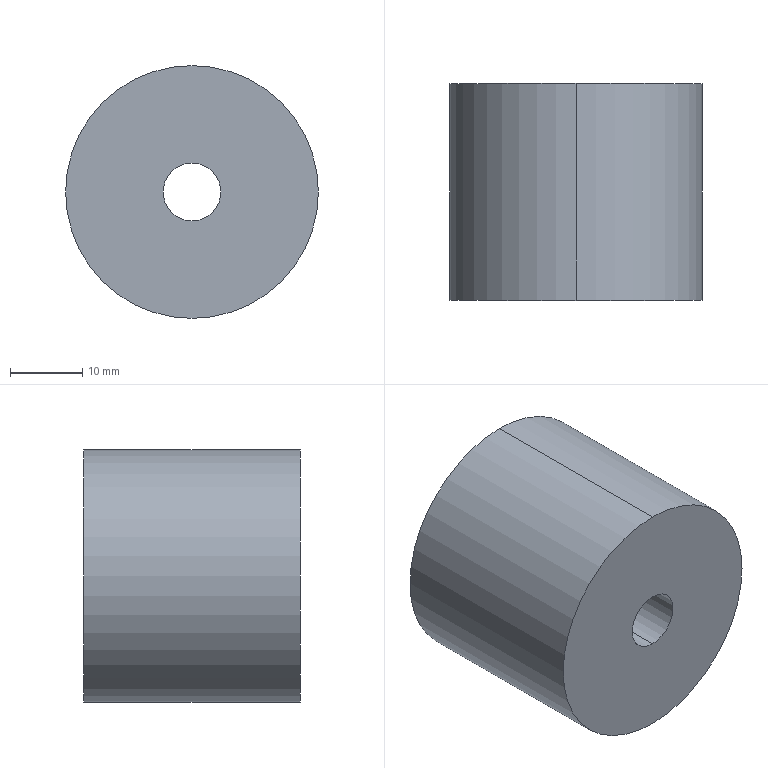Part | STEP file | Polyurethane anti-collision column 2 | 1 solid | 9 faces | box 35 x 30 x 35 mm | volume 26422 mm3 | cylinder 6 | plane 3 | commonest cylinder face diameters 8 x2 14 x2 35 x2
STEP:
#1=CARTESIAN_POINT('',(0.,0.,0.));
#2=DIRECTION('',(0.,0.,1.));
#3=DIRECTION('',(1.,0.,0.));
#4=AXIS2_PLACEMENT_3D('',#1,#2,#3);
#5=CARTESIAN_POINT('',(0.,21.,7.));
#6=VERTEX_POINT('',#5);
#7=CARTESIAN_POINT('',(0.,30.,7.));
#8=VERTEX_POINT('',#7);
#9=CARTESIAN_POINT('',(0.,30.,7.));
#10=DIRECTION('',(0.,1.,0.));
#11=VECTOR('',#10,1.);
#12=LINE('',#9,#11);
#13=CARTESIAN_POINT('',(0.,30.,0.));
#14=DIRECTION('',(0.,1.,0.));
#15=DIRECTION('',(0.,0.,1.));
#16=AXIS2_PLACEMENT_3D('',#13,#14,#15);
#17=CYLINDRICAL_SURFACE('',#16,7.);
#18=CARTESIAN_POINT('',(6.283,0.));
#19=DIRECTION('',(0.,1.));
#20=VECTOR('',#19,1.);
#21=LINE('',#18,#20);
#22=(GEOMETRIC_REPRESENTATION_CONTEXT(2)PARAMETRIC_REPRESENTATION_CONTEXT()REPRESENTATION_CONTEXT('',''));
#23=DEFINITIONAL_REPRESENTATION('',(#21),#22);
#24=PCURVE('',#17,#23);
#25=CARTESIAN_POINT('',(0.,30.,0.));
#26=DIRECTION('',(0.,1.,0.));
#27=DIRECTION('',(0.,0.,1.));
#28=AXIS2_PLACEMENT_3D('',#25,#26,#27);
#29=CYLINDRICAL_SURFACE('',#28,7.);
#30=CARTESIAN_POINT('',(0.,0.));
#31=DIRECTION('',(0.,1.));
#32=VECTOR('',#31,1.);
#33=LINE('',#30,#32);
#34=(GEOMETRIC_REPRESENTATION_CONTEXT(2)PARAMETRIC_REPRESENTATION_CONTEXT()REPRESENTATION_CONTEXT('',''));
#35=DEFINITIONAL_REPRESENTATION('',(#33),#34);
#36=PCURVE('',#29,#35);
#37=SURFACE_CURVE('',#12,(#24,#36),.PCURVE_S1.);
#38=EDGE_CURVE('',#6,#8,#37,.T.);
#39=ORIENTED_EDGE('',*,*,#38,.T.);
#40=CARTESIAN_POINT('',(0.,30.,-7.));
#41=VERTEX_POINT('',#40);
#42=CARTESIAN_POINT('',(0.,30.,0.));
#43=DIRECTION('',(0.,1.,0.));
#44=DIRECTION('',(0.,0.,1.));
#45=AXIS2_PLACEMENT_3D('',#42,#43,#44);
#46=CIRCLE('',#45,7.);
#47=CARTESIAN_POINT('',(0.,0.));
#48=DIRECTION('',(1.,0.));
#49=VECTOR('',#48,1.);
#50=LINE('',#47,#49);
#51=(GEOMETRIC_REPRESENTATION_CONTEXT(2)PARAMETRIC_REPRESENTATION_CONTEXT()REPRESENTATION_CONTEXT('',''));
#52=DEFINITIONAL_REPRESENTATION('',(#50),#51);
#53=PCURVE('',#17,#52);
#54=CARTESIAN_POINT('',(0.,30.,0.));
#55=DIRECTION('',(0.,1.,0.));
#56=DIRECTION('',(0.,0.,1.));
#57=AXIS2_PLACEMENT_3D('',#54,#55,#56);
#58=PLANE('',#57);
#59=CARTESIAN_POINT('',(0.,0.));
#60=DIRECTION('',(1.,0.));
#61=AXIS2_PLACEMENT_2D('',#59,#60);
#62=CIRCLE('',#61,7.);
#63=(GEOMETRIC_REPRESENTATION_CONTEXT(2)PARAMETRIC_REPRESENTATION_CONTEXT()REPRESENTATION_CONTEXT('',''));
#64=DEFINITIONAL_REPRESENTATION('',(#62),#63);
#65=PCURVE('',#58,#64);
#66=SURFACE_CURVE('',#46,(#53,#65),.PCURVE_S1.);
#67=EDGE_CURVE('',#41,#8,#66,.T.);
#68=ORIENTED_EDGE('',*,*,#67,.F.);
#69=CARTESIAN_POINT('',(0.,21.,-7.));
#70=VERTEX_POINT('',#69);
#71=CARTESIAN_POINT('',(0.,30.,-7.));
#72=DIRECTION('',(0.,1.,0.));
#73=VECTOR('',#72,1.);
#74=LINE('',#71,#73);
#75=CARTESIAN_POINT('',(3.142,0.));
#76=DIRECTION('',(0.,1.));
#77=VECTOR('',#76,1.);
#78=LINE('',#75,#77);
#79=(GEOMETRIC_REPRESENTATION_CONTEXT(2)PARAMETRIC_REPRESENTATION_CONTEXT()REPRESENTATION_CONTEXT('',''));
#80=DEFINITIONAL_REPRESENTATION('',(#78),#79);
#81=PCURVE('',#17,#80);
#82=CARTESIAN_POINT('',(3.142,0.));
#83=DIRECTION('',(0.,1.));
#84=VECTOR('',#83,1.);
#85=LINE('',#82,#84);
#86=(GEOMETRIC_REPRESENTATION_CONTEXT(2)PARAMETRIC_REPRESENTATION_CONTEXT()REPRESENTATION_CONTEXT('',''));
#87=DEFINITIONAL_REPRESENTATION('',(#85),#86);
#88=PCURVE('',#29,#87);
#89=SURFACE_CURVE('',#74,(#81,#88),.PCURVE_S1.);
#90=EDGE_CURVE('',#70,#41,#89,.T.);
#91=ORIENTED_EDGE('',*,*,#90,.F.);
#92=CARTESIAN_POINT('',(0.,21.,0.));
#93=DIRECTION('',(0.,1.,0.));
#94=DIRECTION('',(0.,0.,1.));
#95=AXIS2_PLACEMENT_3D('',#92,#93,#94);
#96=CIRCLE('',#95,7.);
#97=CARTESIAN_POINT('',(0.,-9.));
#98=DIRECTION('',(1.,0.));
#99=VECTOR('',#98,1.);
#100=LINE('',#97,#99);
#101=(GEOMETRIC_REPRESENTATION_CONTEXT(2)PARAMETRIC_REPRESENTATION_CONTEXT()REPRESENTATION_CONTEXT('',''));
#102=DEFINITIONAL_REPRESENTATION('',(#100),#101);
#103=PCURVE('',#17,#102);
#104=CARTESIAN_POINT('',(4.,21.,0.));
#105=DIRECTION('',(0.,-1.,0.));
#106=DIRECTION('',(0.,0.,-1.));
#107=AXIS2_PLACEMENT_3D('',#104,#105,#106);
#108=PLANE('',#107);
#109=CARTESIAN_POINT('',(-7.,-4.));
#110=CARTESIAN_POINT('',(-7.,8.124));
#111=CARTESIAN_POINT('',(3.5,2.062));
#112=CARTESIAN_POINT('',(14.,-4.));
#113=CARTESIAN_POINT('',(3.5,-10.062));
#114=CARTESIAN_POINT('',(-7.,-16.124));
#115=CARTESIAN_POINT('',(-7.,-4.));
#116=(BOUNDED_CURVE()B_SPLINE_CURVE(2,(#109,#110,#111,#112,#113,#114,#115),.UNSPECIFIED.,.T.,.F.)B_SPLINE_CURVE_WITH_KNOTS((1,2,2,2,2,1),(-2.094,0.,2.094,4.189,6.283,8.378),.UNSPECIFIED.)CURVE()GEOMETRIC_REPRESENTATION_ITEM()RATIONAL_B_SPLINE_CURVE((1.,0.5,1.,0.5,1.,0.5,1.))REPRESENTATION_ITEM(''));
#117=(GEOMETRIC_REPRESENTATION_CONTEXT(2)PARAMETRIC_REPRESENTATION_CONTEXT()REPRESENTATION_CONTEXT('',''));
#118=DEFINITIONAL_REPRESENTATION('',(#116),#117);
#119=PCURVE('',#108,#118);
#120=SURFACE_CURVE('',#96,(#103,#119),.PCURVE_S1.);
#121=EDGE_CURVE('',#70,#6,#120,.T.);
#122=ORIENTED_EDGE('',*,*,#121,.T.);
#123=EDGE_LOOP('',(#39,#68,#91,#122));
#124=FACE_BOUND('',#123,.F.);
#125=ADVANCED_FACE('',(#124),#17,.F.);
#126=CARTESIAN_POINT('',(0.,0.,4.));
#127=VERTEX_POINT('',#126);
#128=CARTESIAN_POINT('',(0.,21.,4.));
#129=VERTEX_POINT('',#128);
#130=CARTESIAN_POINT('',(0.,30.,4.));
#131=DIRECTION('',(0.,1.,0.));
#132=VECTOR('',#131,1.);
#133=LINE('',#130,#132);
#134=CARTESIAN_POINT('',(0.,30.,0.));
#135=DIRECTION('',(0.,1.,0.));
#136=DIRECTION('',(0.,0.,1.));
#137=AXIS2_PLACEMENT_3D('',#134,#135,#136);
#138=CYLINDRICAL_SURFACE('',#137,4.);
#139=CARTESIAN_POINT('',(6.283,0.));
#140=DIRECTION('',(0.,1.));
#141=VECTOR('',#140,1.);
#142=LINE('',#139,#141);
#143=(GEOMETRIC_REPRESENTATION_CONTEXT(2)PARAMETRIC_REPRESENTATION_CONTEXT()REPRESENTATION_CONTEXT('',''));
#144=DEFINITIONAL_REPRESENTATION('',(#142),#143);
#145=PCURVE('',#138,#144);
#146=CARTESIAN_POINT('',(0.,30.,0.));
#147=DIRECTION('',(0.,1.,0.));
#148=DIRECTION('',(0.,0.,1.));
#149=AXIS2_PLACEMENT_3D('',#146,#147,#148);
#150=CYLINDRICAL_SURFACE('',#149,4.);
#151=CARTESIAN_POINT('',(0.,0.));
#152=DIRECTION('',(0.,1.));
#153=VECTOR('',#152,1.);
#154=LINE('',#151,#153);
#155=(GEOMETRIC_REPRESENTATION_CONTEXT(2)PARAMETRIC_REPRESENTATION_CONTEXT()REPRESENTATION_CONTEXT('',''));
#156=DEFINITIONAL_REPRESENTATION('',(#154),#155);
#157=PCURVE('',#150,#156);
#158=SURFACE_CURVE('',#133,(#145,#157),.PCURVE_S1.);
#159=EDGE_CURVE('',#127,#129,#158,.T.);
#160=ORIENTED_EDGE('',*,*,#159,.T.);
#161=CARTESIAN_POINT('',(0.,21.,-4.));
#162=VERTEX_POINT('',#161);
#163=CARTESIAN_POINT('',(0.,21.,0.));
#164=DIRECTION('',(0.,1.,0.));
#165=DIRECTION('',(0.,0.,1.));
#166=AXIS2_PLACEMENT_3D('',#163,#164,#165);
#167=CIRCLE('',#166,4.);
#168=CARTESIAN_POINT('',(0.,-9.));
#169=DIRECTION('',(1.,0.));
#170=VECTOR('',#169,1.);
#171=LINE('',#168,#170);
#172=(GEOMETRIC_REPRESENTATION_CONTEXT(2)PARAMETRIC_REPRESENTATION_CONTEXT()REPRESENTATION_CONTEXT('',''));
#173=DEFINITIONAL_REPRESENTATION('',(#171),#172);
#174=PCURVE('',#138,#173);
#175=CARTESIAN_POINT('',(-4.,-4.));
#176=CARTESIAN_POINT('',(-4.,2.928));
#177=CARTESIAN_POINT('',(2.,-0.5359));
#178=CARTESIAN_POINT('',(8.,-4.));
#179=CARTESIAN_POINT('',(2.,-7.464));
#180=CARTESIAN_POINT('',(-4.,-10.928));
#181=CARTESIAN_POINT('',(-4.,-4.));
#182=(BOUNDED_CURVE()B_SPLINE_CURVE(2,(#175,#176,#177,#178,#179,#180,#181),.UNSPECIFIED.,.T.,.F.)B_SPLINE_CURVE_WITH_KNOTS((1,2,2,2,2,1),(-2.094,0.,2.094,4.189,6.283,8.378),.UNSPECIFIED.)CURVE()GEOMETRIC_REPRESENTATION_ITEM()RATIONAL_B_SPLINE_CURVE((1.,0.5,1.,0.5,1.,0.5,1.))REPRESENTATION_ITEM(''));
#183=(GEOMETRIC_REPRESENTATION_CONTEXT(2)PARAMETRIC_REPRESENTATION_CONTEXT()REPRESENTATION_CONTEXT('',''));
#184=DEFINITIONAL_REPRESENTATION('',(#182),#183);
#185=PCURVE('',#108,#184);
#186=SURFACE_CURVE('',#167,(#174,#185),.PCURVE_S1.);
#187=EDGE_CURVE('',#162,#129,#186,.T.);
#188=ORIENTED_EDGE('',*,*,#187,.F.);
#189=CARTESIAN_POINT('',(0.,0.,-4.));
#190=VERTEX_POINT('',#189);
#191=CARTESIAN_POINT('',(0.,30.,-4.));
#192=DIRECTION('',(0.,1.,0.));
#193=VECTOR('',#192,1.);
#194=LINE('',#191,#193);
#195=CARTESIAN_POINT('',(3.142,0.));
#196=DIRECTION('',(0.,1.));
#197=VECTOR('',#196,1.);
#198=LINE('',#195,#197);
#199=(GEOMETRIC_REPRESENTATION_CONTEXT(2)PARAMETRIC_REPRESENTATION_CONTEXT()REPRESENTATION_CONTEXT('',''));
#200=DEFINITIONAL_REPRESENTATION('',(#198),#199);
#201=PCURVE('',#138,#200);
#202=CARTESIAN_POINT('',(3.142,0.));
#203=DIRECTION('',(0.,1.));
#204=VECTOR('',#203,1.);
#205=LINE('',#202,#204);
#206=(GEOMETRIC_REPRESENTATION_CONTEXT(2)PARAMETRIC_REPRESENTATION_CONTEXT()REPRESENTATION_CONTEXT('',''));
#207=DEFINITIONAL_REPRESENTATION('',(#205),#206);
#208=PCURVE('',#150,#207);
#209=SURFACE_CURVE('',#194,(#201,#208),.PCURVE_S1.);
#210=EDGE_CURVE('',#190,#162,#209,.T.);
#211=ORIENTED_EDGE('',*,*,#210,.F.);
#212=CARTESIAN_POINT('',(0.,0.,0.));
#213=DIRECTION('',(0.,1.,0.));
#214=DIRECTION('',(0.,0.,1.));
#215=AXIS2_PLACEMENT_3D('',#212,#213,#214);
#216=CIRCLE('',#215,4.);
#217=CARTESIAN_POINT('',(0.,-30.));
#218=DIRECTION('',(1.,0.));
#219=VECTOR('',#218,1.);
#220=LINE('',#217,#219);
#221=(GEOMETRIC_REPRESENTATION_CONTEXT(2)PARAMETRIC_REPRESENTATION_CONTEXT()REPRESENTATION_CONTEXT('',''));
#222=DEFINITIONAL_REPRESENTATION('',(#220),#221);
#223=PCURVE('',#138,#222);
#224=CARTESIAN_POINT('',(0.,0.,0.));
#225=DIRECTION('',(0.,1.,0.));
#226=DIRECTION('',(0.,0.,1.));
#227=AXIS2_PLACEMENT_3D('',#224,#225,#226);
#228=PLANE('',#227);
#229=CARTESIAN_POINT('',(0.,0.));
#230=DIRECTION('',(1.,0.));
#231=AXIS2_PLACEMENT_2D('',#229,#230);
#232=CIRCLE('',#231,4.);
#233=(GEOMETRIC_REPRESENTATION_CONTEXT(2)PARAMETRIC_REPRESENTATION_CONTEXT()REPRESENTATION_CONTEXT('',''));
#234=DEFINITIONAL_REPRESENTATION('',(#232),#233);
#235=PCURVE('',#228,#234);
#236=SURFACE_CURVE('',#216,(#223,#235),.PCURVE_S1.);
#237=EDGE_CURVE('',#190,#127,#236,.T.);
#238=ORIENTED_EDGE('',*,*,#237,.T.);
#239=EDGE_LOOP('',(#160,#188,#211,#238));
#240=FACE_BOUND('',#239,.F.);
#241=ADVANCED_FACE('',(#240),#138,.F.);
#242=CARTESIAN_POINT('',(0.,30.,17.5));
#243=VERTEX_POINT('',#242);
#244=CARTESIAN_POINT('',(0.,30.,-17.5));
#245=VERTEX_POINT('',#244);
#246=CARTESIAN_POINT('',(0.,30.,0.));
#247=DIRECTION('',(0.,1.,0.));
#248=DIRECTION('',(0.,0.,1.));
#249=AXIS2_PLACEMENT_3D('',#246,#247,#248);
#250=CIRCLE('',#249,17.5);
#251=CARTESIAN_POINT('',(0.,30.,0.));
#252=DIRECTION('',(0.,-1.,0.));
#253=DIRECTION('',(0.,0.,-1.));
#254=AXIS2_PLACEMENT_3D('',#251,#252,#253);
#255=CYLINDRICAL_SURFACE('',#254,17.5);
#256=CARTESIAN_POINT('',(3.142,0.));
#257=DIRECTION('',(-1.,0.));
#258=VECTOR('',#257,1.);
#259=LINE('',#256,#258);
#260=(GEOMETRIC_REPRESENTATION_CONTEXT(2)PARAMETRIC_REPRESENTATION_CONTEXT()REPRESENTATION_CONTEXT('',''));
#261=DEFINITIONAL_REPRESENTATION('',(#259),#260);
#262=PCURVE('',#255,#261);
#263=CARTESIAN_POINT('',(0.,0.));
#264=DIRECTION('',(1.,0.));
#265=AXIS2_PLACEMENT_2D('',#263,#264);
#266=CIRCLE('',#265,17.5);
#267=(GEOMETRIC_REPRESENTATION_CONTEXT(2)PARAMETRIC_REPRESENTATION_CONTEXT()REPRESENTATION_CONTEXT('',''));
#268=DEFINITIONAL_REPRESENTATION('',(#266),#267);
#269=PCURVE('',#58,#268);
#270=SURFACE_CURVE('',#250,(#262,#269),.PCURVE_S1.);
#271=EDGE_CURVE('',#243,#245,#270,.T.);
#272=ORIENTED_EDGE('',*,*,#271,.F.);
#273=CARTESIAN_POINT('',(0.,0.,17.5));
#274=VERTEX_POINT('',#273);
#275=CARTESIAN_POINT('',(0.,30.,17.5));
#276=DIRECTION('',(0.,-1.,0.));
#277=VECTOR('',#276,1.);
#278=LINE('',#275,#277);
#279=CARTESIAN_POINT('',(3.142,0.));
#280=DIRECTION('',(0.,1.));
#281=VECTOR('',#280,1.);
#282=LINE('',#279,#281);
#283=(GEOMETRIC_REPRESENTATION_CONTEXT(2)PARAMETRIC_REPRESENTATION_CONTEXT()REPRESENTATION_CONTEXT('',''));
#284=DEFINITIONAL_REPRESENTATION('',(#282),#283);
#285=PCURVE('',#255,#284);
#286=CARTESIAN_POINT('',(0.,30.,0.));
#287=DIRECTION('',(0.,-1.,0.));
#288=DIRECTION('',(0.,0.,-1.));
#289=AXIS2_PLACEMENT_3D('',#286,#287,#288);
#290=CYLINDRICAL_SURFACE('',#289,17.5);
#291=CARTESIAN_POINT('',(3.142,0.));
#292=DIRECTION('',(0.,1.));
#293=VECTOR('',#292,1.);
#294=LINE('',#291,#293);
#295=(GEOMETRIC_REPRESENTATION_CONTEXT(2)PARAMETRIC_REPRESENTATION_CONTEXT()REPRESENTATION_CONTEXT('',''));
#296=DEFINITIONAL_REPRESENTATION('',(#294),#295);
#297=PCURVE('',#290,#296);
#298=SURFACE_CURVE('',#278,(#285,#297),.PCURVE_S1.);
#299=EDGE_CURVE('',#243,#274,#298,.T.);
#300=ORIENTED_EDGE('',*,*,#299,.T.);
#301=CARTESIAN_POINT('',(0.,0.,-17.5));
#302=VERTEX_POINT('',#301);
#303=CARTESIAN_POINT('',(0.,0.,0.));
#304=DIRECTION('',(0.,1.,0.));
#305=DIRECTION('',(0.,0.,1.));
#306=AXIS2_PLACEMENT_3D('',#303,#304,#305);
#307=CIRCLE('',#306,17.5);
#308=CARTESIAN_POINT('',(3.142,30.));
#309=DIRECTION('',(-1.,0.));
#310=VECTOR('',#309,1.);
#311=LINE('',#308,#310);
#312=(GEOMETRIC_REPRESENTATION_CONTEXT(2)PARAMETRIC_REPRESENTATION_CONTEXT()REPRESENTATION_CONTEXT('',''));
#313=DEFINITIONAL_REPRESENTATION('',(#311),#312);
#314=PCURVE('',#255,#313);
#315=CARTESIAN_POINT('',(0.,0.));
#316=DIRECTION('',(1.,0.));
#317=AXIS2_PLACEMENT_2D('',#315,#316);
#318=CIRCLE('',#317,17.5);
#319=(GEOMETRIC_REPRESENTATION_CONTEXT(2)PARAMETRIC_REPRESENTATION_CONTEXT()REPRESENTATION_CONTEXT('',''));
#320=DEFINITIONAL_REPRESENTATION('',(#318),#319);
#321=PCURVE('',#228,#320);
#322=SURFACE_CURVE('',#307,(#314,#321),.PCURVE_S1.);
#323=EDGE_CURVE('',#274,#302,#322,.T.);
#324=ORIENTED_EDGE('',*,*,#323,.T.);
#325=CARTESIAN_POINT('',(0.,30.,-17.5));
#326=DIRECTION('',(0.,-1.,0.));
#327=VECTOR('',#326,1.);
#328=LINE('',#325,#327);
#329=CARTESIAN_POINT('',(0.,0.));
#330=DIRECTION('',(0.,1.));
#331=VECTOR('',#330,1.);
#332=LINE('',#329,#331);
#333=(GEOMETRIC_REPRESENTATION_CONTEXT(2)PARAMETRIC_REPRESENTATION_CONTEXT()REPRESENTATION_CONTEXT('',''));
#334=DEFINITIONAL_REPRESENTATION('',(#332),#333);
#335=PCURVE('',#255,#334);
#336=CARTESIAN_POINT('',(6.283,0.));
#337=DIRECTION('',(0.,1.));
#338=VECTOR('',#337,1.);
#339=LINE('',#336,#338);
#340=(GEOMETRIC_REPRESENTATION_CONTEXT(2)PARAMETRIC_REPRESENTATION_CONTEXT()REPRESENTATION_CONTEXT('',''));
#341=DEFINITIONAL_REPRESENTATION('',(#339),#340);
#342=PCURVE('',#290,#341);
#343=SURFACE_CURVE('',#328,(#335,#342),.PCURVE_S1.);
#344=EDGE_CURVE('',#245,#302,#343,.T.);
#345=ORIENTED_EDGE('',*,*,#344,.F.);
#346=EDGE_LOOP('',(#272,#300,#324,#345));
#347=FACE_BOUND('',#346,.T.);
#348=ADVANCED_FACE('',(#347),#255,.T.);
#349=ORIENTED_EDGE('',*,*,#299,.F.);
#350=CARTESIAN_POINT('',(0.,30.,0.));
#351=DIRECTION('',(0.,1.,0.));
#352=DIRECTION('',(0.,0.,1.));
#353=AXIS2_PLACEMENT_3D('',#350,#351,#352);
#354=CIRCLE('',#353,17.5);
#355=CARTESIAN_POINT('',(9.425,0.));
#356=DIRECTION('',(-1.,0.));
#357=VECTOR('',#356,1.);
#358=LINE('',#355,#357);
#359=(GEOMETRIC_REPRESENTATION_CONTEXT(2)PARAMETRIC_REPRESENTATION_CONTEXT()REPRESENTATION_CONTEXT('',''));
#360=DEFINITIONAL_REPRESENTATION('',(#358),#359);
#361=PCURVE('',#290,#360);
#362=CARTESIAN_POINT('',(0.,0.));
#363=DIRECTION('',(1.,0.));
#364=AXIS2_PLACEMENT_2D('',#362,#363);
#365=CIRCLE('',#364,17.5);
#366=(GEOMETRIC_REPRESENTATION_CONTEXT(2)PARAMETRIC_REPRESENTATION_CONTEXT()REPRESENTATION_CONTEXT('',''));
#367=DEFINITIONAL_REPRESENTATION('',(#365),#366);
#368=PCURVE('',#58,#367);
#369=SURFACE_CURVE('',#354,(#361,#368),.PCURVE_S1.);
#370=EDGE_CURVE('',#245,#243,#369,.T.);
#371=ORIENTED_EDGE('',*,*,#370,.F.);
#372=ORIENTED_EDGE('',*,*,#344,.T.);
#373=CARTESIAN_POINT('',(0.,0.,0.));
#374=DIRECTION('',(0.,1.,0.));
#375=DIRECTION('',(0.,0.,1.));
#376=AXIS2_PLACEMENT_3D('',#373,#374,#375);
#377=CIRCLE('',#376,17.5);
#378=CARTESIAN_POINT('',(9.425,30.));
#379=DIRECTION('',(-1.,0.));
#380=VECTOR('',#379,1.);
#381=LINE('',#378,#380);
#382=(GEOMETRIC_REPRESENTATION_CONTEXT(2)PARAMETRIC_REPRESENTATION_CONTEXT()REPRESENTATION_CONTEXT('',''));
#383=DEFINITIONAL_REPRESENTATION('',(#381),#382);
#384=PCURVE('',#290,#383);
#385=CARTESIAN_POINT('',(0.,0.));
#386=DIRECTION('',(1.,0.));
#387=AXIS2_PLACEMENT_2D('',#385,#386);
#388=CIRCLE('',#387,17.5);
#389=(GEOMETRIC_REPRESENTATION_CONTEXT(2)PARAMETRIC_REPRESENTATION_CONTEXT()REPRESENTATION_CONTEXT('',''));
#390=DEFINITIONAL_REPRESENTATION('',(#388),#389);
#391=PCURVE('',#228,#390);
#392=SURFACE_CURVE('',#377,(#384,#391),.PCURVE_S1.);
#393=EDGE_CURVE('',#302,#274,#392,.T.);
#394=ORIENTED_EDGE('',*,*,#393,.T.);
#395=EDGE_LOOP('',(#349,#371,#372,#394));
#396=FACE_BOUND('',#395,.T.);
#397=ADVANCED_FACE('',(#396),#290,.T.);
#398=CARTESIAN_POINT('',(0.,30.,0.));
#399=DIRECTION('',(0.,1.,0.));
#400=DIRECTION('',(0.,0.,1.));
#401=AXIS2_PLACEMENT_3D('',#398,#399,#400);
#402=CIRCLE('',#401,7.);
#403=CARTESIAN_POINT('',(0.,0.));
#404=DIRECTION('',(1.,0.));
#405=AXIS2_PLACEMENT_2D('',#403,#404);
#406=CIRCLE('',#405,7.);
#407=(GEOMETRIC_REPRESENTATION_CONTEXT(2)PARAMETRIC_REPRESENTATION_CONTEXT()REPRESENTATION_CONTEXT('',''));
#408=DEFINITIONAL_REPRESENTATION('',(#406),#407);
#409=PCURVE('',#58,#408);
#410=CARTESIAN_POINT('',(0.,0.));
#411=DIRECTION('',(1.,0.));
#412=VECTOR('',#411,1.);
#413=LINE('',#410,#412);
#414=(GEOMETRIC_REPRESENTATION_CONTEXT(2)PARAMETRIC_REPRESENTATION_CONTEXT()REPRESENTATION_CONTEXT('',''));
#415=DEFINITIONAL_REPRESENTATION('',(#413),#414);
#416=PCURVE('',#29,#415);
#417=SURFACE_CURVE('',#402,(#409,#416),.PCURVE_S1.);
#418=EDGE_CURVE('',#8,#41,#417,.T.);
#419=ORIENTED_EDGE('',*,*,#418,.F.);
#420=ORIENTED_EDGE('',*,*,#67,.F.);
#421=EDGE_LOOP('',(#419,#420));
#422=FACE_BOUND('',#421,.T.);
#423=ORIENTED_EDGE('',*,*,#370,.T.);
#424=ORIENTED_EDGE('',*,*,#271,.T.);
#425=EDGE_LOOP('',(#423,#424));
#426=FACE_BOUND('',#425,.T.);
#427=ADVANCED_FACE('',(#422,#426),#58,.T.);
#428=CARTESIAN_POINT('',(0.,0.,0.));
#429=DIRECTION('',(0.,1.,0.));
#430=DIRECTION('',(0.,0.,1.));
#431=AXIS2_PLACEMENT_3D('',#428,#429,#430);
#432=CIRCLE('',#431,4.);
#433=CARTESIAN_POINT('',(0.,0.));
#434=DIRECTION('',(1.,0.));
#435=AXIS2_PLACEMENT_2D('',#433,#434);
#436=CIRCLE('',#435,4.);
#437=(GEOMETRIC_REPRESENTATION_CONTEXT(2)PARAMETRIC_REPRESENTATION_CONTEXT()REPRESENTATION_CONTEXT('',''));
#438=DEFINITIONAL_REPRESENTATION('',(#436),#437);
#439=PCURVE('',#228,#438);
#440=CARTESIAN_POINT('',(0.,-30.));
#441=DIRECTION('',(1.,0.));
#442=VECTOR('',#441,1.);
#443=LINE('',#440,#442);
#444=(GEOMETRIC_REPRESENTATION_CONTEXT(2)PARAMETRIC_REPRESENTATION_CONTEXT()REPRESENTATION_CONTEXT('',''));
#445=DEFINITIONAL_REPRESENTATION('',(#443),#444);
#446=PCURVE('',#150,#445);
#447=SURFACE_CURVE('',#432,(#439,#446),.PCURVE_S1.);
#448=EDGE_CURVE('',#127,#190,#447,.T.);
#449=ORIENTED_EDGE('',*,*,#448,.T.);
#450=ORIENTED_EDGE('',*,*,#237,.T.);
#451=EDGE_LOOP('',(#449,#450));
#452=FACE_BOUND('',#451,.T.);
#453=ORIENTED_EDGE('',*,*,#393,.F.);
#454=ORIENTED_EDGE('',*,*,#323,.F.);
#455=EDGE_LOOP('',(#453,#454));
#456=FACE_BOUND('',#455,.T.);
#457=ADVANCED_FACE('',(#452,#456),#228,.F.);
#458=CARTESIAN_POINT('',(0.,21.,0.));
#459=DIRECTION('',(0.,1.,0.));
#460=DIRECTION('',(0.,0.,1.));
#461=AXIS2_PLACEMENT_3D('',#458,#459,#460);
#462=CIRCLE('',#461,4.);
#463=CARTESIAN_POINT('',(0.,-9.));
#464=DIRECTION('',(1.,0.));
#465=VECTOR('',#464,1.);
#466=LINE('',#463,#465);
#467=(GEOMETRIC_REPRESENTATION_CONTEXT(2)PARAMETRIC_REPRESENTATION_CONTEXT()REPRESENTATION_CONTEXT('',''));
#468=DEFINITIONAL_REPRESENTATION('',(#466),#467);
#469=PCURVE('',#150,#468);
#470=CARTESIAN_POINT('',(-4.,-4.));
#471=CARTESIAN_POINT('',(-4.,2.928));
#472=CARTESIAN_POINT('',(2.,-0.5359));
#473=CARTESIAN_POINT('',(8.,-4.));
#474=CARTESIAN_POINT('',(2.,-7.464));
#475=CARTESIAN_POINT('',(-4.,-10.928));
#476=CARTESIAN_POINT('',(-4.,-4.));
#477=(BOUNDED_CURVE()B_SPLINE_CURVE(2,(#470,#471,#472,#473,#474,#475,#476),.UNSPECIFIED.,.T.,.F.)B_SPLINE_CURVE_WITH_KNOTS((1,2,2,2,2,1),(-2.094,0.,2.094,4.189,6.283,8.378),.UNSPECIFIED.)CURVE()GEOMETRIC_REPRESENTATION_ITEM()RATIONAL_B_SPLINE_CURVE((1.,0.5,1.,0.5,1.,0.5,1.))REPRESENTATION_ITEM(''));
#478=(GEOMETRIC_REPRESENTATION_CONTEXT(2)PARAMETRIC_REPRESENTATION_CONTEXT()REPRESENTATION_CONTEXT('',''));
#479=DEFINITIONAL_REPRESENTATION('',(#477),#478);
#480=PCURVE('',#108,#479);
#481=SURFACE_CURVE('',#462,(#469,#480),.PCURVE_S1.);
#482=EDGE_CURVE('',#129,#162,#481,.T.);
#483=ORIENTED_EDGE('',*,*,#482,.F.);
#484=ORIENTED_EDGE('',*,*,#159,.F.);
#485=ORIENTED_EDGE('',*,*,#448,.T.);
#486=ORIENTED_EDGE('',*,*,#210,.T.);
#487=EDGE_LOOP('',(#483,#484,#485,#486));
#488=FACE_BOUND('',#487,.F.);
#489=ADVANCED_FACE('',(#488),#150,.F.);
#490=ORIENTED_EDGE('',*,*,#482,.F.);
#491=ORIENTED_EDGE('',*,*,#187,.F.);
#492=EDGE_LOOP('',(#490,#491));
#493=FACE_BOUND('',#492,.T.);
#494=CARTESIAN_POINT('',(0.,21.,0.));
#495=DIRECTION('',(0.,1.,0.));
#496=DIRECTION('',(0.,0.,1.));
#497=AXIS2_PLACEMENT_3D('',#494,#495,#496);
#498=CIRCLE('',#497,7.);
#499=CARTESIAN_POINT('',(-7.,-4.));
#500=CARTESIAN_POINT('',(-7.,8.124));
#501=CARTESIAN_POINT('',(3.5,2.062));
#502=CARTESIAN_POINT('',(14.,-4.));
#503=CARTESIAN_POINT('',(3.5,-10.062));
#504=CARTESIAN_POINT('',(-7.,-16.124));
#505=CARTESIAN_POINT('',(-7.,-4.));
#506=(BOUNDED_CURVE()B_SPLINE_CURVE(2,(#499,#500,#501,#502,#503,#504,#505),.UNSPECIFIED.,.T.,.F.)B_SPLINE_CURVE_WITH_KNOTS((1,2,2,2,2,1),(-2.094,0.,2.094,4.189,6.283,8.378),.UNSPECIFIED.)CURVE()GEOMETRIC_REPRESENTATION_ITEM()RATIONAL_B_SPLINE_CURVE((1.,0.5,1.,0.5,1.,0.5,1.))REPRESENTATION_ITEM(''));
#507=(GEOMETRIC_REPRESENTATION_CONTEXT(2)PARAMETRIC_REPRESENTATION_CONTEXT()REPRESENTATION_CONTEXT('',''));
#508=DEFINITIONAL_REPRESENTATION('',(#506),#507);
#509=PCURVE('',#108,#508);
#510=CARTESIAN_POINT('',(0.,-9.));
#511=DIRECTION('',(1.,0.));
#512=VECTOR('',#511,1.);
#513=LINE('',#510,#512);
#514=(GEOMETRIC_REPRESENTATION_CONTEXT(2)PARAMETRIC_REPRESENTATION_CONTEXT()REPRESENTATION_CONTEXT('',''));
#515=DEFINITIONAL_REPRESENTATION('',(#513),#514);
#516=PCURVE('',#29,#515);
#517=SURFACE_CURVE('',#498,(#509,#516),.PCURVE_S1.);
#518=EDGE_CURVE('',#6,#70,#517,.T.);
#519=ORIENTED_EDGE('',*,*,#518,.T.);
#520=ORIENTED_EDGE('',*,*,#121,.T.);
#521=EDGE_LOOP('',(#519,#520));
#522=FACE_BOUND('',#521,.T.);
#523=ADVANCED_FACE('',(#493,#522),#108,.F.);
#524=ORIENTED_EDGE('',*,*,#418,.F.);
#525=ORIENTED_EDGE('',*,*,#38,.F.);
#526=ORIENTED_EDGE('',*,*,#518,.T.);
#527=ORIENTED_EDGE('',*,*,#90,.T.);
#528=EDGE_LOOP('',(#524,#525,#526,#527));
#529=FACE_BOUND('',#528,.F.);
#530=ADVANCED_FACE('',(#529),#29,.F.);
#531=CLOSED_SHELL('',(#125,#241,#348,#397,#427,#457,#489,#523,#530));
#532=MANIFOLD_SOLID_BREP('',#531);
#533=(LENGTH_UNIT()NAMED_UNIT(*)SI_UNIT(.MILLI.,.METRE.));
#534=UNCERTAINTY_MEASURE_WITH_UNIT(LENGTH_MEASURE(0.0000001),#533,'','');
#535=(NAMED_UNIT(*)PLANE_ANGLE_UNIT()SI_UNIT($,.RADIAN.));
#536=(NAMED_UNIT(*)SI_UNIT($,.STERADIAN.)SOLID_ANGLE_UNIT());
#537=(GEOMETRIC_REPRESENTATION_CONTEXT(3)GLOBAL_UNCERTAINTY_ASSIGNED_CONTEXT((#534))GLOBAL_UNIT_ASSIGNED_CONTEXT((#533,#535,#536))REPRESENTATION_CONTEXT('',''));
#538=ADVANCED_BREP_SHAPE_REPRESENTATION('',(#4,#532),#537);